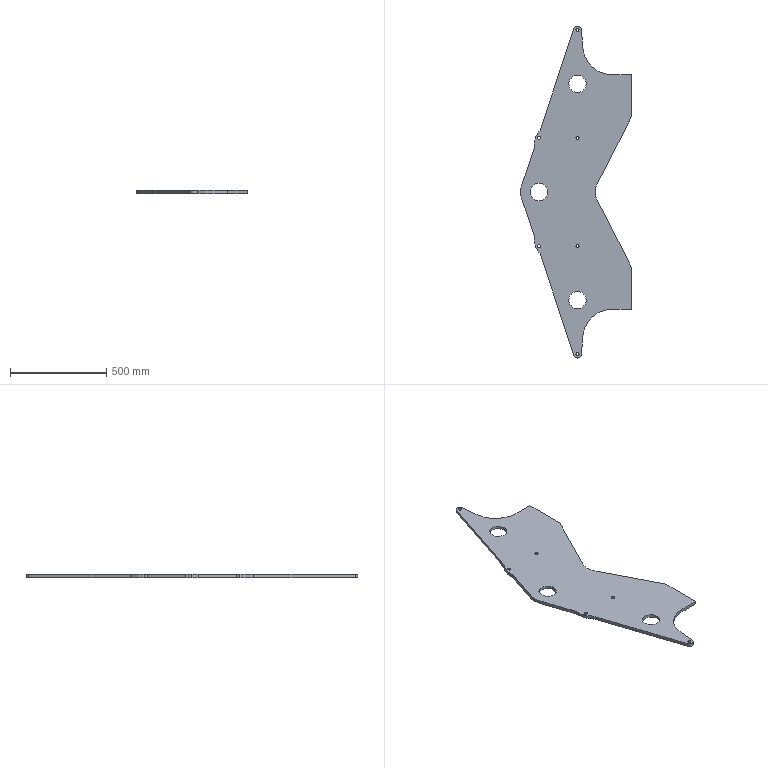Part | SolidWorks | features Extrusion 1, HoleWzd 1, ICE 1 | 1 solid | 44 faces | box 575.631 x 1726 x 16 mm | volume 8635461 mm3 | cylinder 30 | plane 14 | commonest cylinder face diameters 16 x12 200 x8 90 x6 40 x2 300 x2
STEP:
#1=CARTESIAN_POINT('',(-503.404,233.68,16.));
#2=VERTEX_POINT('',#1);
#3=CARTESIAN_POINT('',(-504.662,249.486,16.));
#4=VERTEX_POINT('',#3);
#5=CARTESIAN_POINT('',(-404.662,249.486,16.));
#6=DIRECTION('',(0.,0.,-1.));
#7=DIRECTION('',(1.,0.,0.));
#8=AXIS2_PLACEMENT_3D('',#5,#6,#7);
#9=CIRCLE('',#8,100.);
#10=EDGE_CURVE('',#2,#4,#9,.T.);
#11=ORIENTED_EDGE('',*,*,#10,.T.);
#12=CARTESIAN_POINT('',(-504.662,249.486,0.));
#13=VERTEX_POINT('',#12);
#14=CARTESIAN_POINT('',(-504.662,249.486,16.));
#15=DIRECTION('',(0.,0.,-1.));
#16=VECTOR('',#15,1000.);
#17=LINE('',#14,#16);
#18=EDGE_CURVE('',#4,#13,#17,.T.);
#19=ORIENTED_EDGE('',*,*,#18,.T.);
#20=CARTESIAN_POINT('',(-503.404,233.68,0.));
#21=VERTEX_POINT('',#20);
#22=CARTESIAN_POINT('',(-404.662,249.486,0.));
#23=DIRECTION('',(0.,0.,-1.));
#24=DIRECTION('',(1.,0.,0.));
#25=AXIS2_PLACEMENT_3D('',#22,#23,#24);
#26=CIRCLE('',#25,100.);
#27=EDGE_CURVE('',#21,#13,#26,.T.);
#28=ORIENTED_EDGE('',*,*,#27,.F.);
#29=CARTESIAN_POINT('',(-503.404,233.68,16.));
#30=DIRECTION('',(0.,0.,-1.));
#31=VECTOR('',#30,1000.);
#32=LINE('',#29,#31);
#33=EDGE_CURVE('',#2,#21,#32,.T.);
#34=ORIENTED_EDGE('',*,*,#33,.F.);
#35=EDGE_LOOP('',(#11,#19,#28,#34));
#36=FACE_OUTER_BOUND('',#35,.T.);
#37=CARTESIAN_POINT('',(-404.662,249.486,16.));
#38=DIRECTION('',(0.,0.,-1.));
#39=DIRECTION('',(-1.,0.,0.));
#40=AXIS2_PLACEMENT_3D('',#37,#38,#39);
#41=CYLINDRICAL_SURFACE('',#40,100.);
#42=ADVANCED_FACE('',(#36),#41,.T.);
#43=CARTESIAN_POINT('',(-235.,562.,16.));
#44=VERTEX_POINT('',#43);
#45=CARTESIAN_POINT('',(-325.,562.,16.));
#46=VERTEX_POINT('',#45);
#47=CARTESIAN_POINT('',(-280.,562.,16.));
#48=DIRECTION('',(0.,0.,-1.));
#49=DIRECTION('',(1.,0.,0.));
#50=AXIS2_PLACEMENT_3D('',#47,#48,#49);
#51=CIRCLE('',#50,45.);
#52=EDGE_CURVE('',#44,#46,#51,.T.);
#53=ORIENTED_EDGE('',*,*,#52,.F.);
#54=CARTESIAN_POINT('',(-235.,562.,0.));
#55=VERTEX_POINT('',#54);
#56=CARTESIAN_POINT('',(-235.,562.,16.));
#57=DIRECTION('',(0.,0.,-1.));
#58=VECTOR('',#57,1000.);
#59=LINE('',#56,#58);
#60=EDGE_CURVE('',#44,#55,#59,.T.);
#61=ORIENTED_EDGE('',*,*,#60,.T.);
#62=CARTESIAN_POINT('',(-325.,562.,0.));
#63=VERTEX_POINT('',#62);
#64=CARTESIAN_POINT('',(-280.,562.,0.));
#65=DIRECTION('',(0.,0.,-1.));
#66=DIRECTION('',(1.,0.,0.));
#67=AXIS2_PLACEMENT_3D('',#64,#65,#66);
#68=CIRCLE('',#67,45.);
#69=EDGE_CURVE('',#55,#63,#68,.T.);
#70=ORIENTED_EDGE('',*,*,#69,.T.);
#71=CARTESIAN_POINT('',(-325.,562.,16.));
#72=DIRECTION('',(0.,0.,-1.));
#73=VECTOR('',#72,1000.);
#74=LINE('',#71,#73);
#75=EDGE_CURVE('',#46,#63,#74,.T.);
#76=ORIENTED_EDGE('',*,*,#75,.F.);
#77=EDGE_LOOP('',(#53,#61,#70,#76));
#78=FACE_OUTER_BOUND('',#77,.T.);
#79=CARTESIAN_POINT('',(-280.,562.,16.));
#80=DIRECTION('',(0.,0.,-1.));
#81=DIRECTION('',(-1.,0.,0.));
#82=AXIS2_PLACEMENT_3D('',#79,#80,#81);
#83=CYLINDRICAL_SURFACE('',#82,45.);
#84=ADVANCED_FACE('',(#78),#83,.F.);
#85=CARTESIAN_POINT('',(-272.,281.,16.));
#86=VERTEX_POINT('',#85);
#87=CARTESIAN_POINT('',(-288.,281.,16.));
#88=VERTEX_POINT('',#87);
#89=CARTESIAN_POINT('',(-280.,281.,16.));
#90=DIRECTION('',(0.,0.,-1.));
#91=DIRECTION('',(1.,0.,0.));
#92=AXIS2_PLACEMENT_3D('',#89,#90,#91);
#93=CIRCLE('',#92,8.);
#94=EDGE_CURVE('',#86,#88,#93,.T.);
#95=ORIENTED_EDGE('',*,*,#94,.F.);
#96=CARTESIAN_POINT('',(-272.,281.,0.));
#97=VERTEX_POINT('',#96);
#98=CARTESIAN_POINT('',(-272.,281.,16.));
#99=DIRECTION('',(0.,0.,-1.));
#100=VECTOR('',#99,1000.);
#101=LINE('',#98,#100);
#102=EDGE_CURVE('',#86,#97,#101,.T.);
#103=ORIENTED_EDGE('',*,*,#102,.T.);
#104=CARTESIAN_POINT('',(-288.,281.,0.));
#105=VERTEX_POINT('',#104);
#106=CARTESIAN_POINT('',(-280.,281.,0.));
#107=DIRECTION('',(0.,0.,-1.));
#108=DIRECTION('',(1.,0.,0.));
#109=AXIS2_PLACEMENT_3D('',#106,#107,#108);
#110=CIRCLE('',#109,8.);
#111=EDGE_CURVE('',#97,#105,#110,.T.);
#112=ORIENTED_EDGE('',*,*,#111,.T.);
#113=CARTESIAN_POINT('',(-288.,281.,16.));
#114=DIRECTION('',(0.,0.,-1.));
#115=VECTOR('',#114,1000.);
#116=LINE('',#113,#115);
#117=EDGE_CURVE('',#88,#105,#116,.T.);
#118=ORIENTED_EDGE('',*,*,#117,.F.);
#119=EDGE_LOOP('',(#95,#103,#112,#118));
#120=FACE_OUTER_BOUND('',#119,.T.);
#121=CARTESIAN_POINT('',(-280.,281.,16.));
#122=DIRECTION('',(0.,0.,-1.));
#123=DIRECTION('',(-1.,0.,0.));
#124=AXIS2_PLACEMENT_3D('',#121,#122,#123);
#125=CYLINDRICAL_SURFACE('',#124,8.);
#126=ADVANCED_FACE('',(#120),#125,.F.);
#127=CARTESIAN_POINT('',(-288.,843.,16.));
#128=VERTEX_POINT('',#127);
#129=CARTESIAN_POINT('',(-272.,843.,16.));
#130=VERTEX_POINT('',#129);
#131=CARTESIAN_POINT('',(-280.,843.,16.));
#132=DIRECTION('',(0.,0.,1.));
#133=DIRECTION('',(1.,0.,0.));
#134=AXIS2_PLACEMENT_3D('',#131,#132,#133);
#135=CIRCLE('',#134,8.);
#136=EDGE_CURVE('',#128,#130,#135,.T.);
#137=ORIENTED_EDGE('',*,*,#136,.T.);
#138=CARTESIAN_POINT('',(-272.,843.,0.));
#139=VERTEX_POINT('',#138);
#140=CARTESIAN_POINT('',(-272.,843.,16.));
#141=DIRECTION('',(0.,0.,-1.));
#142=VECTOR('',#141,1000.);
#143=LINE('',#140,#142);
#144=EDGE_CURVE('',#130,#139,#143,.T.);
#145=ORIENTED_EDGE('',*,*,#144,.T.);
#146=CARTESIAN_POINT('',(-288.,843.,0.));
#147=VERTEX_POINT('',#146);
#148=CARTESIAN_POINT('',(-280.,843.,0.));
#149=DIRECTION('',(0.,0.,1.));
#150=DIRECTION('',(1.,0.,0.));
#151=AXIS2_PLACEMENT_3D('',#148,#149,#150);
#152=CIRCLE('',#151,8.);
#153=EDGE_CURVE('',#147,#139,#152,.T.);
#154=ORIENTED_EDGE('',*,*,#153,.F.);
#155=CARTESIAN_POINT('',(-288.,843.,16.));
#156=DIRECTION('',(0.,0.,-1.));
#157=VECTOR('',#156,1000.);
#158=LINE('',#155,#157);
#159=EDGE_CURVE('',#128,#147,#158,.T.);
#160=ORIENTED_EDGE('',*,*,#159,.F.);
#161=EDGE_LOOP('',(#137,#145,#154,#160));
#162=FACE_OUTER_BOUND('',#161,.T.);
#163=CARTESIAN_POINT('',(-280.,843.,16.));
#164=DIRECTION('',(0.,0.,-1.));
#165=DIRECTION('',(-1.,0.,0.));
#166=AXIS2_PLACEMENT_3D('',#163,#164,#165);
#167=CYLINDRICAL_SURFACE('',#166,8.);
#168=ADVANCED_FACE('',(#162),#167,.F.);
#169=CARTESIAN_POINT('',(-288.,-843.,16.));
#170=VERTEX_POINT('',#169);
#171=CARTESIAN_POINT('',(-272.,-843.,16.));
#172=VERTEX_POINT('',#171);
#173=CARTESIAN_POINT('',(-280.,-843.,16.));
#174=DIRECTION('',(0.,0.,1.));
#175=DIRECTION('',(1.,0.,0.));
#176=AXIS2_PLACEMENT_3D('',#173,#174,#175);
#177=CIRCLE('',#176,8.);
#178=EDGE_CURVE('',#170,#172,#177,.T.);
#179=ORIENTED_EDGE('',*,*,#178,.T.);
#180=CARTESIAN_POINT('',(-272.,-843.,0.));
#181=VERTEX_POINT('',#180);
#182=CARTESIAN_POINT('',(-272.,-843.,16.));
#183=DIRECTION('',(0.,0.,-1.));
#184=VECTOR('',#183,1000.);
#185=LINE('',#182,#184);
#186=EDGE_CURVE('',#172,#181,#185,.T.);
#187=ORIENTED_EDGE('',*,*,#186,.T.);
#188=CARTESIAN_POINT('',(-288.,-843.,0.));
#189=VERTEX_POINT('',#188);
#190=CARTESIAN_POINT('',(-280.,-843.,0.));
#191=DIRECTION('',(0.,0.,1.));
#192=DIRECTION('',(1.,0.,0.));
#193=AXIS2_PLACEMENT_3D('',#190,#191,#192);
#194=CIRCLE('',#193,8.);
#195=EDGE_CURVE('',#189,#181,#194,.T.);
#196=ORIENTED_EDGE('',*,*,#195,.F.);
#197=CARTESIAN_POINT('',(-288.,-843.,16.));
#198=DIRECTION('',(0.,0.,-1.));
#199=VECTOR('',#198,1000.);
#200=LINE('',#197,#199);
#201=EDGE_CURVE('',#170,#189,#200,.T.);
#202=ORIENTED_EDGE('',*,*,#201,.F.);
#203=EDGE_LOOP('',(#179,#187,#196,#202));
#204=FACE_OUTER_BOUND('',#203,.T.);
#205=CARTESIAN_POINT('',(-280.,-843.,16.));
#206=DIRECTION('',(0.,0.,-1.));
#207=DIRECTION('',(-1.,0.,0.));
#208=AXIS2_PLACEMENT_3D('',#205,#206,#207);
#209=CYLINDRICAL_SURFACE('',#208,8.);
#210=ADVANCED_FACE('',(#204),#209,.F.);
#211=CARTESIAN_POINT('',(-288.,-281.,16.));
#212=VERTEX_POINT('',#211);
#213=CARTESIAN_POINT('',(-272.,-281.,16.));
#214=VERTEX_POINT('',#213);
#215=CARTESIAN_POINT('',(-280.,-281.,16.));
#216=DIRECTION('',(0.,0.,1.));
#217=DIRECTION('',(1.,0.,0.));
#218=AXIS2_PLACEMENT_3D('',#215,#216,#217);
#219=CIRCLE('',#218,8.);
#220=EDGE_CURVE('',#212,#214,#219,.T.);
#221=ORIENTED_EDGE('',*,*,#220,.T.);
#222=CARTESIAN_POINT('',(-272.,-281.,0.));
#223=VERTEX_POINT('',#222);
#224=CARTESIAN_POINT('',(-272.,-281.,16.));
#225=DIRECTION('',(0.,0.,-1.));
#226=VECTOR('',#225,1000.);
#227=LINE('',#224,#226);
#228=EDGE_CURVE('',#214,#223,#227,.T.);
#229=ORIENTED_EDGE('',*,*,#228,.T.);
#230=CARTESIAN_POINT('',(-288.,-281.,0.));
#231=VERTEX_POINT('',#230);
#232=CARTESIAN_POINT('',(-280.,-281.,0.));
#233=DIRECTION('',(0.,0.,1.));
#234=DIRECTION('',(1.,0.,0.));
#235=AXIS2_PLACEMENT_3D('',#232,#233,#234);
#236=CIRCLE('',#235,8.);
#237=EDGE_CURVE('',#231,#223,#236,.T.);
#238=ORIENTED_EDGE('',*,*,#237,.F.);
#239=CARTESIAN_POINT('',(-288.,-281.,16.));
#240=DIRECTION('',(0.,0.,-1.));
#241=VECTOR('',#240,1000.);
#242=LINE('',#239,#241);
#243=EDGE_CURVE('',#212,#231,#242,.T.);
#244=ORIENTED_EDGE('',*,*,#243,.F.);
#245=EDGE_LOOP('',(#221,#229,#238,#244));
#246=FACE_OUTER_BOUND('',#245,.T.);
#247=CARTESIAN_POINT('',(-280.,-281.,16.));
#248=DIRECTION('',(0.,0.,-1.));
#249=DIRECTION('',(-1.,0.,0.));
#250=AXIS2_PLACEMENT_3D('',#247,#248,#249);
#251=CYLINDRICAL_SURFACE('',#250,8.);
#252=ADVANCED_FACE('',(#246),#251,.F.);
#253=CARTESIAN_POINT('',(-488.,-281.,16.));
#254=VERTEX_POINT('',#253);
#255=CARTESIAN_POINT('',(-472.,-281.,16.));
#256=VERTEX_POINT('',#255);
#257=CARTESIAN_POINT('',(-480.,-281.,16.));
#258=DIRECTION('',(0.,0.,1.));
#259=DIRECTION('',(1.,0.,0.));
#260=AXIS2_PLACEMENT_3D('',#257,#258,#259);
#261=CIRCLE('',#260,8.);
#262=EDGE_CURVE('',#254,#256,#261,.T.);
#263=ORIENTED_EDGE('',*,*,#262,.T.);
#264=CARTESIAN_POINT('',(-472.,-281.,0.));
#265=VERTEX_POINT('',#264);
#266=CARTESIAN_POINT('',(-472.,-281.,16.));
#267=DIRECTION('',(0.,0.,-1.));
#268=VECTOR('',#267,1000.);
#269=LINE('',#266,#268);
#270=EDGE_CURVE('',#256,#265,#269,.T.);
#271=ORIENTED_EDGE('',*,*,#270,.T.);
#272=CARTESIAN_POINT('',(-488.,-281.,0.));
#273=VERTEX_POINT('',#272);
#274=CARTESIAN_POINT('',(-480.,-281.,0.));
#275=DIRECTION('',(0.,0.,1.));
#276=DIRECTION('',(1.,0.,0.));
#277=AXIS2_PLACEMENT_3D('',#274,#275,#276);
#278=CIRCLE('',#277,8.);
#279=EDGE_CURVE('',#273,#265,#278,.T.);
#280=ORIENTED_EDGE('',*,*,#279,.F.);
#281=CARTESIAN_POINT('',(-488.,-281.,16.));
#282=DIRECTION('',(0.,0.,-1.));
#283=VECTOR('',#282,1000.);
#284=LINE('',#281,#283);
#285=EDGE_CURVE('',#254,#273,#284,.T.);
#286=ORIENTED_EDGE('',*,*,#285,.F.);
#287=EDGE_LOOP('',(#263,#271,#280,#286));
#288=FACE_OUTER_BOUND('',#287,.T.);
#289=CARTESIAN_POINT('',(-480.,-281.,16.));
#290=DIRECTION('',(0.,0.,-1.));
#291=DIRECTION('',(-1.,0.,0.));
#292=AXIS2_PLACEMENT_3D('',#289,#290,#291);
#293=CYLINDRICAL_SURFACE('',#292,8.);
#294=ADVANCED_FACE('',(#288),#293,.F.);
#295=CARTESIAN_POINT('',(-325.,-562.,16.));
#296=VERTEX_POINT('',#295);
#297=CARTESIAN_POINT('',(-235.,-562.,16.));
#298=VERTEX_POINT('',#297);
#299=CARTESIAN_POINT('',(-280.,-562.,16.));
#300=DIRECTION('',(0.,0.,1.));
#301=DIRECTION('',(1.,0.,0.));
#302=AXIS2_PLACEMENT_3D('',#299,#300,#301);
#303=CIRCLE('',#302,45.);
#304=EDGE_CURVE('',#296,#298,#303,.T.);
#305=ORIENTED_EDGE('',*,*,#304,.T.);
#306=CARTESIAN_POINT('',(-235.,-562.,0.));
#307=VERTEX_POINT('',#306);
#308=CARTESIAN_POINT('',(-235.,-562.,16.));
#309=DIRECTION('',(0.,0.,-1.));
#310=VECTOR('',#309,1000.);
#311=LINE('',#308,#310);
#312=EDGE_CURVE('',#298,#307,#311,.T.);
#313=ORIENTED_EDGE('',*,*,#312,.T.);
#314=CARTESIAN_POINT('',(-325.,-562.,0.));
#315=VERTEX_POINT('',#314);
#316=CARTESIAN_POINT('',(-280.,-562.,0.));
#317=DIRECTION('',(0.,0.,1.));
#318=DIRECTION('',(1.,0.,0.));
#319=AXIS2_PLACEMENT_3D('',#316,#317,#318);
#320=CIRCLE('',#319,45.);
#321=EDGE_CURVE('',#315,#307,#320,.T.);
#322=ORIENTED_EDGE('',*,*,#321,.F.);
#323=CARTESIAN_POINT('',(-325.,-562.,16.));
#324=DIRECTION('',(0.,0.,-1.));
#325=VECTOR('',#324,1000.);
#326=LINE('',#323,#325);
#327=EDGE_CURVE('',#296,#315,#326,.T.);
#328=ORIENTED_EDGE('',*,*,#327,.F.);
#329=EDGE_LOOP('',(#305,#313,#322,#328));
#330=FACE_OUTER_BOUND('',#329,.T.);
#331=CARTESIAN_POINT('',(-280.,-562.,16.));
#332=DIRECTION('',(0.,0.,-1.));
#333=DIRECTION('',(-1.,0.,0.));
#334=AXIS2_PLACEMENT_3D('',#331,#332,#333);
#335=CYLINDRICAL_SURFACE('',#334,45.);
#336=ADVANCED_FACE('',(#330),#335,.F.);
#337=CARTESIAN_POINT('',(-525.,0.,16.));
#338=VERTEX_POINT('',#337);
#339=CARTESIAN_POINT('',(-435.,0.,16.));
#340=VERTEX_POINT('',#339);
#341=CARTESIAN_POINT('',(-480.,0.,16.));
#342=DIRECTION('',(0.,0.,1.));
#343=DIRECTION('',(1.,0.,0.));
#344=AXIS2_PLACEMENT_3D('',#341,#342,#343);
#345=CIRCLE('',#344,45.);
#346=EDGE_CURVE('',#338,#340,#345,.T.);
#347=ORIENTED_EDGE('',*,*,#346,.T.);
#348=CARTESIAN_POINT('',(-435.,0.,0.));
#349=VERTEX_POINT('',#348);
#350=CARTESIAN_POINT('',(-435.,0.,16.));
#351=DIRECTION('',(0.,0.,-1.));
#352=VECTOR('',#351,1000.);
#353=LINE('',#350,#352);
#354=EDGE_CURVE('',#340,#349,#353,.T.);
#355=ORIENTED_EDGE('',*,*,#354,.T.);
#356=CARTESIAN_POINT('',(-525.,0.,0.));
#357=VERTEX_POINT('',#356);
#358=CARTESIAN_POINT('',(-480.,0.,0.));
#359=DIRECTION('',(0.,0.,1.));
#360=DIRECTION('',(1.,0.,0.));
#361=AXIS2_PLACEMENT_3D('',#358,#359,#360);
#362=CIRCLE('',#361,45.);
#363=EDGE_CURVE('',#357,#349,#362,.T.);
#364=ORIENTED_EDGE('',*,*,#363,.F.);
#365=CARTESIAN_POINT('',(-525.,0.,16.));
#366=DIRECTION('',(0.,0.,-1.));
#367=VECTOR('',#366,1000.);
#368=LINE('',#365,#367);
#369=EDGE_CURVE('',#338,#357,#368,.T.);
#370=ORIENTED_EDGE('',*,*,#369,.F.);
#371=EDGE_LOOP('',(#347,#355,#364,#370));
#372=FACE_OUTER_BOUND('',#371,.T.);
#373=CARTESIAN_POINT('',(-480.,0.,16.));
#374=DIRECTION('',(0.,0.,-1.));
#375=DIRECTION('',(-1.,0.,0.));
#376=AXIS2_PLACEMENT_3D('',#373,#374,#375);
#377=CYLINDRICAL_SURFACE('',#376,45.);
#378=ADVANCED_FACE('',(#372),#377,.F.);
#379=CARTESIAN_POINT('',(-472.,281.,16.));
#380=VERTEX_POINT('',#379);
#381=CARTESIAN_POINT('',(-488.,281.,16.));
#382=VERTEX_POINT('',#381);
#383=CARTESIAN_POINT('',(-480.,281.,16.));
#384=DIRECTION('',(0.,0.,-1.));
#385=DIRECTION('',(1.,0.,0.));
#386=AXIS2_PLACEMENT_3D('',#383,#384,#385);
#387=CIRCLE('',#386,8.);
#388=EDGE_CURVE('',#380,#382,#387,.T.);
#389=ORIENTED_EDGE('',*,*,#388,.F.);
#390=CARTESIAN_POINT('',(-472.,281.,0.));
#391=VERTEX_POINT('',#390);
#392=CARTESIAN_POINT('',(-472.,281.,16.));
#393=DIRECTION('',(0.,0.,-1.));
#394=VECTOR('',#393,1000.);
#395=LINE('',#392,#394);
#396=EDGE_CURVE('',#380,#391,#395,.T.);
#397=ORIENTED_EDGE('',*,*,#396,.T.);
#398=CARTESIAN_POINT('',(-488.,281.,0.));
#399=VERTEX_POINT('',#398);
#400=CARTESIAN_POINT('',(-480.,281.,0.));
#401=DIRECTION('',(0.,0.,-1.));
#402=DIRECTION('',(1.,0.,0.));
#403=AXIS2_PLACEMENT_3D('',#400,#401,#402);
#404=CIRCLE('',#403,8.);
#405=EDGE_CURVE('',#391,#399,#404,.T.);
#406=ORIENTED_EDGE('',*,*,#405,.T.);
#407=CARTESIAN_POINT('',(-488.,281.,16.));
#408=DIRECTION('',(0.,0.,-1.));
#409=VECTOR('',#408,1000.);
#410=LINE('',#407,#409);
#411=EDGE_CURVE('',#382,#399,#410,.T.);
#412=ORIENTED_EDGE('',*,*,#411,.F.);
#413=EDGE_LOOP('',(#389,#397,#406,#412));
#414=FACE_OUTER_BOUND('',#413,.T.);
#415=CARTESIAN_POINT('',(-480.,281.,16.));
#416=DIRECTION('',(0.,0.,-1.));
#417=DIRECTION('',(-1.,0.,0.));
#418=AXIS2_PLACEMENT_3D('',#415,#416,#417);
#419=CYLINDRICAL_SURFACE('',#418,8.);
#420=ADVANCED_FACE('',(#414),#419,.F.);
#421=CARTESIAN_POINT('',(-176.599,45.632,16.));
#422=VERTEX_POINT('',#421);
#423=CARTESIAN_POINT('',(-187.617,0.,16.));
#424=VERTEX_POINT('',#423);
#425=CARTESIAN_POINT('',(-87.617,0.,16.));
#426=DIRECTION('',(0.,0.,1.));
#427=DIRECTION('',(1.,0.,0.));
#428=AXIS2_PLACEMENT_3D('',#425,#426,#427);
#429=CIRCLE('',#428,100.);
#430=EDGE_CURVE('',#422,#424,#429,.T.);
#431=ORIENTED_EDGE('',*,*,#430,.T.);
#432=CARTESIAN_POINT('',(-187.617,0.,0.));
#433=VERTEX_POINT('',#432);
#434=CARTESIAN_POINT('',(-187.617,0.,16.));
#435=DIRECTION('',(0.,0.,-1.));
#436=VECTOR('',#435,1000.);
#437=LINE('',#434,#436);
#438=EDGE_CURVE('',#424,#433,#437,.T.);
#439=ORIENTED_EDGE('',*,*,#438,.T.);
#440=CARTESIAN_POINT('',(-176.599,45.632,0.));
#441=VERTEX_POINT('',#440);
#442=CARTESIAN_POINT('',(-87.617,0.,0.));
#443=DIRECTION('',(0.,0.,1.));
#444=DIRECTION('',(1.,0.,0.));
#445=AXIS2_PLACEMENT_3D('',#442,#443,#444);
#446=CIRCLE('',#445,100.);
#447=EDGE_CURVE('',#441,#433,#446,.T.);
#448=ORIENTED_EDGE('',*,*,#447,.F.);
#449=CARTESIAN_POINT('',(-176.599,45.632,16.));
#450=DIRECTION('',(0.,0.,-1.));
#451=VECTOR('',#450,1000.);
#452=LINE('',#449,#451);
#453=EDGE_CURVE('',#422,#441,#452,.T.);
#454=ORIENTED_EDGE('',*,*,#453,.F.);
#455=EDGE_LOOP('',(#431,#439,#448,#454));
#456=FACE_OUTER_BOUND('',#455,.T.);
#457=CARTESIAN_POINT('',(-87.617,0.,16.));
#458=DIRECTION('',(0.,0.,-1.));
#459=DIRECTION('',(-1.,0.,0.));
#460=AXIS2_PLACEMENT_3D('',#457,#458,#459);
#461=CYLINDRICAL_SURFACE('',#460,100.);
#462=ADVANCED_FACE('',(#456),#461,.F.);
#463=CARTESIAN_POINT('',(-504.662,-249.486,16.));
#464=VERTEX_POINT('',#463);
#465=CARTESIAN_POINT('',(-474.337,-321.217,16.));
#466=VERTEX_POINT('',#465);
#467=CARTESIAN_POINT('',(-404.662,-249.486,16.));
#468=DIRECTION('',(0.,0.,1.));
#469=DIRECTION('',(1.,0.,0.));
#470=AXIS2_PLACEMENT_3D('',#467,#468,#469);
#471=CIRCLE('',#470,100.);
#472=EDGE_CURVE('',#464,#466,#471,.T.);
#473=ORIENTED_EDGE('',*,*,#472,.F.);
#474=CARTESIAN_POINT('',(-504.662,-249.486,0.));
#475=VERTEX_POINT('',#474);
#476=CARTESIAN_POINT('',(-504.662,-249.486,16.));
#477=DIRECTION('',(0.,0.,-1.));
#478=VECTOR('',#477,1000.);
#479=LINE('',#476,#478);
#480=EDGE_CURVE('',#464,#475,#479,.T.);
#481=ORIENTED_EDGE('',*,*,#480,.T.);
#482=CARTESIAN_POINT('',(-474.337,-321.217,0.));
#483=VERTEX_POINT('',#482);
#484=CARTESIAN_POINT('',(-404.662,-249.486,0.));
#485=DIRECTION('',(0.,0.,1.));
#486=DIRECTION('',(1.,0.,0.));
#487=AXIS2_PLACEMENT_3D('',#484,#485,#486);
#488=CIRCLE('',#487,100.);
#489=EDGE_CURVE('',#475,#483,#488,.T.);
#490=ORIENTED_EDGE('',*,*,#489,.T.);
#491=CARTESIAN_POINT('',(-474.337,-321.217,16.));
#492=DIRECTION('',(0.,0.,-1.));
#493=VECTOR('',#492,1000.);
#494=LINE('',#491,#493);
#495=EDGE_CURVE('',#466,#483,#494,.T.);
#496=ORIENTED_EDGE('',*,*,#495,.F.);
#497=EDGE_LOOP('',(#473,#481,#490,#496));
#498=FACE_OUTER_BOUND('',#497,.T.);
#499=CARTESIAN_POINT('',(-404.662,-249.486,16.));
#500=DIRECTION('',(0.,0.,-1.));
#501=DIRECTION('',(-1.,0.,0.));
#502=AXIS2_PLACEMENT_3D('',#499,#500,#501);
#503=CYLINDRICAL_SURFACE('',#502,100.);
#504=ADVANCED_FACE('',(#498),#503,.T.);
#505=CARTESIAN_POINT('',(-575.631,0.,16.));
#506=VERTEX_POINT('',#505);
#507=CARTESIAN_POINT('',(-570.535,-31.514,16.));
#508=VERTEX_POINT('',#507);
#509=CARTESIAN_POINT('',(-475.631,0.,16.));
#510=DIRECTION('',(0.,0.,1.));
#511=DIRECTION('',(1.,0.,0.));
#512=AXIS2_PLACEMENT_3D('',#509,#510,#511);
#513=CIRCLE('',#512,100.);
#514=EDGE_CURVE('',#506,#508,#513,.T.);
#515=ORIENTED_EDGE('',*,*,#514,.F.);
#516=CARTESIAN_POINT('',(-575.631,0.,0.));
#517=VERTEX_POINT('',#516);
#518=CARTESIAN_POINT('',(-575.631,0.,16.));
#519=DIRECTION('',(0.,0.,-1.));
#520=VECTOR('',#519,1000.);
#521=LINE('',#518,#520);
#522=EDGE_CURVE('',#506,#517,#521,.T.);
#523=ORIENTED_EDGE('',*,*,#522,.T.);
#524=CARTESIAN_POINT('',(-570.535,-31.514,0.));
#525=VERTEX_POINT('',#524);
#526=CARTESIAN_POINT('',(-475.631,0.,0.));
#527=DIRECTION('',(0.,0.,1.));
#528=DIRECTION('',(1.,0.,0.));
#529=AXIS2_PLACEMENT_3D('',#526,#527,#528);
#530=CIRCLE('',#529,100.);
#531=EDGE_CURVE('',#517,#525,#530,.T.);
#532=ORIENTED_EDGE('',*,*,#531,.T.);
#533=CARTESIAN_POINT('',(-570.535,-31.514,16.));
#534=DIRECTION('',(0.,0.,-1.));
#535=VECTOR('',#534,1000.);
#536=LINE('',#533,#535);
#537=EDGE_CURVE('',#508,#525,#536,.T.);
#538=ORIENTED_EDGE('',*,*,#537,.F.);
#539=EDGE_LOOP('',(#515,#523,#532,#538));
#540=FACE_OUTER_BOUND('',#539,.T.);
#541=CARTESIAN_POINT('',(-475.631,0.,16.));
#542=DIRECTION('',(0.,0.,-1.));
#543=DIRECTION('',(-1.,0.,0.));
#544=AXIS2_PLACEMENT_3D('',#541,#542,#543);
#545=CYLINDRICAL_SURFACE('',#544,100.);
#546=ADVANCED_FACE('',(#540),#545,.T.);
#547=CARTESIAN_POINT('',(-570.535,31.514,0.));
#548=VERTEX_POINT('',#547);
#549=CARTESIAN_POINT('',(-523.299,173.766,0.));
#550=DIRECTION('',(0.3151,0.949,0.));
#551=VECTOR('',#550,1000.);
#552=LINE('',#549,#551);
#553=EDGE_CURVE('',#548,#21,#552,.T.);
#554=ORIENTED_EDGE('',*,*,#553,.F.);
#555=CARTESIAN_POINT('',(-570.535,31.514,16.));
#556=VERTEX_POINT('',#555);
#557=CARTESIAN_POINT('',(-570.535,31.514,16.));
#558=DIRECTION('',(0.,0.,-1.));
#559=VECTOR('',#558,1000.);
#560=LINE('',#557,#559);
#561=EDGE_CURVE('',#556,#548,#560,.T.);
#562=ORIENTED_EDGE('',*,*,#561,.F.);
#563=CARTESIAN_POINT('',(-523.299,173.766,16.));
#564=DIRECTION('',(0.3151,0.949,0.));
#565=VECTOR('',#564,1000.);
#566=LINE('',#563,#565);
#567=EDGE_CURVE('',#556,#2,#566,.T.);
#568=ORIENTED_EDGE('',*,*,#567,.T.);
#569=ORIENTED_EDGE('',*,*,#33,.T.);
#570=EDGE_LOOP('',(#554,#562,#568,#569));
#571=FACE_OUTER_BOUND('',#570,.T.);
#572=CARTESIAN_POINT('',(-523.299,173.766,16.));
#573=DIRECTION('',(-0.949,0.3151,0.));
#574=DIRECTION('',(-0.3151,-0.949,0.));
#575=AXIS2_PLACEMENT_3D('',#572,#573,#574);
#576=PLANE('',#575);
#577=ADVANCED_FACE('',(#571),#576,.T.);
#578=ORIENTED_EDGE('',*,*,#522,.F.);
#579=CARTESIAN_POINT('',(-475.631,0.,16.));
#580=DIRECTION('',(0.,0.,1.));
#581=DIRECTION('',(1.,0.,0.));
#582=AXIS2_PLACEMENT_3D('',#579,#580,#581);
#583=CIRCLE('',#582,100.);
#584=EDGE_CURVE('',#556,#506,#583,.T.);
#585=ORIENTED_EDGE('',*,*,#584,.F.);
#586=ORIENTED_EDGE('',*,*,#561,.T.);
#587=CARTESIAN_POINT('',(-475.631,0.,0.));
#588=DIRECTION('',(0.,0.,1.));
#589=DIRECTION('',(1.,0.,0.));
#590=AXIS2_PLACEMENT_3D('',#587,#588,#589);
#591=CIRCLE('',#590,100.);
#592=EDGE_CURVE('',#548,#517,#591,.T.);
#593=ORIENTED_EDGE('',*,*,#592,.T.);
#594=EDGE_LOOP('',(#578,#585,#586,#593));
#595=FACE_OUTER_BOUND('',#594,.T.);
#596=CARTESIAN_POINT('',(-475.631,0.,16.));
#597=DIRECTION('',(0.,0.,-1.));
#598=DIRECTION('',(-1.,0.,0.));
#599=AXIS2_PLACEMENT_3D('',#596,#597,#598);
#600=CYLINDRICAL_SURFACE('',#599,100.);
#601=ADVANCED_FACE('',(#595),#600,.T.);
#602=CARTESIAN_POINT('',(-503.404,-233.68,0.));
#603=VERTEX_POINT('',#602);
#604=CARTESIAN_POINT('',(-523.299,-173.766,0.));
#605=DIRECTION('',(0.3151,-0.949,0.));
#606=VECTOR('',#605,1000.);
#607=LINE('',#604,#606);
#608=EDGE_CURVE('',#525,#603,#607,.T.);
#609=ORIENTED_EDGE('',*,*,#608,.T.);
#610=CARTESIAN_POINT('',(-503.404,-233.68,16.));
#611=VERTEX_POINT('',#610);
#612=CARTESIAN_POINT('',(-503.404,-233.68,16.));
#613=DIRECTION('',(0.,0.,-1.));
#614=VECTOR('',#613,1000.);
#615=LINE('',#612,#614);
#616=EDGE_CURVE('',#611,#603,#615,.T.);
#617=ORIENTED_EDGE('',*,*,#616,.F.);
#618=CARTESIAN_POINT('',(-523.299,-173.766,16.));
#619=DIRECTION('',(0.3151,-0.949,0.));
#620=VECTOR('',#619,1000.);
#621=LINE('',#618,#620);
#622=EDGE_CURVE('',#508,#611,#621,.T.);
#623=ORIENTED_EDGE('',*,*,#622,.F.);
#624=ORIENTED_EDGE('',*,*,#537,.T.);
#625=EDGE_LOOP('',(#609,#617,#623,#624));
#626=FACE_OUTER_BOUND('',#625,.T.);
#627=CARTESIAN_POINT('',(-523.299,-173.766,16.));
#628=DIRECTION('',(0.949,0.3151,0.));
#629=DIRECTION('',(-0.3151,0.949,0.));
#630=AXIS2_PLACEMENT_3D('',#627,#628,#629);
#631=PLANE('',#630);
#632=ADVANCED_FACE('',(#626),#631,.F.);
#633=ORIENTED_EDGE('',*,*,#480,.F.);
#634=CARTESIAN_POINT('',(-404.662,-249.486,16.));
#635=DIRECTION('',(0.,0.,1.));
#636=DIRECTION('',(1.,0.,0.));
#637=AXIS2_PLACEMENT_3D('',#634,#635,#636);
#638=CIRCLE('',#637,100.);
#639=EDGE_CURVE('',#611,#464,#638,.T.);
#640=ORIENTED_EDGE('',*,*,#639,.F.);
#641=ORIENTED_EDGE('',*,*,#616,.T.);
#642=CARTESIAN_POINT('',(-404.662,-249.486,0.));
#643=DIRECTION('',(0.,0.,1.));
#644=DIRECTION('',(1.,0.,0.));
#645=AXIS2_PLACEMENT_3D('',#642,#643,#644);
#646=CIRCLE('',#645,100.);
#647=EDGE_CURVE('',#603,#475,#646,.T.);
#648=ORIENTED_EDGE('',*,*,#647,.T.);
#649=EDGE_LOOP('',(#633,#640,#641,#648));
#650=FACE_OUTER_BOUND('',#649,.T.);
#651=CARTESIAN_POINT('',(-404.662,-249.486,16.));
#652=DIRECTION('',(0.,0.,-1.));
#653=DIRECTION('',(-1.,0.,0.));
#654=AXIS2_PLACEMENT_3D('',#651,#652,#653);
#655=CYLINDRICAL_SURFACE('',#654,100.);
#656=ADVANCED_FACE('',(#650),#655,.T.);
#657=CARTESIAN_POINT('',(-298.981,-849.303,0.));
#658=VERTEX_POINT('',#657);
#659=CARTESIAN_POINT('',(-523.299,-173.766,0.));
#660=DIRECTION('',(0.3151,-0.949,0.));
#661=VECTOR('',#660,1000.);
#662=LINE('',#659,#661);
#663=EDGE_CURVE('',#483,#658,#662,.T.);
#664=ORIENTED_EDGE('',*,*,#663,.T.);
#665=CARTESIAN_POINT('',(-298.981,-849.303,16.));
#666=VERTEX_POINT('',#665);
#667=CARTESIAN_POINT('',(-298.981,-849.303,16.));
#668=DIRECTION('',(0.,0.,-1.));
#669=VECTOR('',#668,1000.);
#670=LINE('',#667,#669);
#671=EDGE_CURVE('',#666,#658,#670,.T.);
#672=ORIENTED_EDGE('',*,*,#671,.F.);
#673=CARTESIAN_POINT('',(-523.299,-173.766,16.));
#674=DIRECTION('',(0.3151,-0.949,0.));
#675=VECTOR('',#674,1000.);
#676=LINE('',#673,#675);
#677=EDGE_CURVE('',#466,#666,#676,.T.);
#678=ORIENTED_EDGE('',*,*,#677,.F.);
#679=ORIENTED_EDGE('',*,*,#495,.T.);
#680=EDGE_LOOP('',(#664,#672,#678,#679));
#681=FACE_OUTER_BOUND('',#680,.T.);
#682=CARTESIAN_POINT('',(-523.299,-173.766,16.));
#683=DIRECTION('',(0.949,0.3151,0.));
#684=DIRECTION('',(-0.3151,0.949,0.));
#685=AXIS2_PLACEMENT_3D('',#682,#683,#684);
#686=PLANE('',#685);
#687=ADVANCED_FACE('',(#681),#686,.F.);
#688=CARTESIAN_POINT('',(-260.076,-844.743,0.));
#689=VERTEX_POINT('',#688);
#690=CARTESIAN_POINT('',(-280.,-843.,0.));
#691=DIRECTION('',(0.,0.,-1.));
#692=DIRECTION('',(1.,0.,0.));
#693=AXIS2_PLACEMENT_3D('',#690,#691,#692);
#694=CIRCLE('',#693,20.);
#695=EDGE_CURVE('',#689,#658,#694,.T.);
#696=ORIENTED_EDGE('',*,*,#695,.F.);
#697=CARTESIAN_POINT('',(-260.076,-844.743,16.));
#698=VERTEX_POINT('',#697);
#699=CARTESIAN_POINT('',(-260.076,-844.743,16.));
#700=DIRECTION('',(0.,0.,-1.));
#701=VECTOR('',#700,1000.);
#702=LINE('',#699,#701);
#703=EDGE_CURVE('',#698,#689,#702,.T.);
#704=ORIENTED_EDGE('',*,*,#703,.F.);
#705=CARTESIAN_POINT('',(-280.,-843.,16.));
#706=DIRECTION('',(0.,0.,-1.));
#707=DIRECTION('',(1.,0.,0.));
#708=AXIS2_PLACEMENT_3D('',#705,#706,#707);
#709=CIRCLE('',#708,20.);
#710=EDGE_CURVE('',#698,#666,#709,.T.);
#711=ORIENTED_EDGE('',*,*,#710,.T.);
#712=ORIENTED_EDGE('',*,*,#671,.T.);
#713=EDGE_LOOP('',(#696,#704,#711,#712));
#714=FACE_OUTER_BOUND('',#713,.T.);
#715=CARTESIAN_POINT('',(-280.,-843.,16.));
#716=DIRECTION('',(0.,0.,-1.));
#717=DIRECTION('',(-1.,0.,0.));
#718=AXIS2_PLACEMENT_3D('',#715,#716,#717);
#719=CYLINDRICAL_SURFACE('',#718,20.);
#720=ADVANCED_FACE('',(#714),#719,.T.);
#721=CARTESIAN_POINT('',(-251.518,-746.927,0.));
#722=VERTEX_POINT('',#721);
#723=CARTESIAN_POINT('',(-184.756,16.164,0.));
#724=DIRECTION('',(0.08716,0.9962,0.));
#725=VECTOR('',#724,1000.);
#726=LINE('',#723,#725);
#727=EDGE_CURVE('',#689,#722,#726,.T.);
#728=ORIENTED_EDGE('',*,*,#727,.T.);
#729=CARTESIAN_POINT('',(-251.518,-746.927,16.));
#730=VERTEX_POINT('',#729);
#731=CARTESIAN_POINT('',(-251.518,-746.927,16.));
#732=DIRECTION('',(0.,0.,-1.));
#733=VECTOR('',#732,1000.);
#734=LINE('',#731,#733);
#735=EDGE_CURVE('',#730,#722,#734,.T.);
#736=ORIENTED_EDGE('',*,*,#735,.F.);
#737=CARTESIAN_POINT('',(-184.756,16.164,16.));
#738=DIRECTION('',(0.08716,0.9962,0.));
#739=VECTOR('',#738,1000.);
#740=LINE('',#737,#739);
#741=EDGE_CURVE('',#698,#730,#740,.T.);
#742=ORIENTED_EDGE('',*,*,#741,.F.);
#743=ORIENTED_EDGE('',*,*,#703,.T.);
#744=EDGE_LOOP('',(#728,#736,#742,#743));
#745=FACE_OUTER_BOUND('',#744,.T.);
#746=CARTESIAN_POINT('',(-184.756,16.164,16.));
#747=DIRECTION('',(-0.9962,0.08716,0.));
#748=DIRECTION('',(-0.08716,-0.9962,0.));
#749=AXIS2_PLACEMENT_3D('',#746,#747,#748);
#750=PLANE('',#749);
#751=ADVANCED_FACE('',(#745),#750,.F.);
#752=CARTESIAN_POINT('',(-102.089,-610.,0.));
#753=VERTEX_POINT('',#752);
#754=CARTESIAN_POINT('',(-102.089,-760.,0.));
#755=DIRECTION('',(0.,0.,1.));
#756=DIRECTION('',(1.,0.,0.));
#757=AXIS2_PLACEMENT_3D('',#754,#755,#756);
#758=CIRCLE('',#757,150.);
#759=EDGE_CURVE('',#753,#722,#758,.T.);
#760=ORIENTED_EDGE('',*,*,#759,.F.);
#761=CARTESIAN_POINT('',(-102.089,-610.,16.));
#762=VERTEX_POINT('',#761);
#763=CARTESIAN_POINT('',(-102.089,-610.,16.));
#764=DIRECTION('',(0.,0.,-1.));
#765=VECTOR('',#764,1000.);
#766=LINE('',#763,#765);
#767=EDGE_CURVE('',#762,#753,#766,.T.);
#768=ORIENTED_EDGE('',*,*,#767,.F.);
#769=CARTESIAN_POINT('',(-102.089,-760.,16.));
#770=DIRECTION('',(0.,0.,1.));
#771=DIRECTION('',(1.,0.,0.));
#772=AXIS2_PLACEMENT_3D('',#769,#770,#771);
#773=CIRCLE('',#772,150.);
#774=EDGE_CURVE('',#762,#730,#773,.T.);
#775=ORIENTED_EDGE('',*,*,#774,.T.);
#776=ORIENTED_EDGE('',*,*,#735,.T.);
#777=EDGE_LOOP('',(#760,#768,#775,#776));
#778=FACE_OUTER_BOUND('',#777,.T.);
#779=CARTESIAN_POINT('',(-102.089,-760.,16.));
#780=DIRECTION('',(0.,0.,-1.));
#781=DIRECTION('',(-1.,0.,0.));
#782=AXIS2_PLACEMENT_3D('',#779,#780,#781);
#783=CYLINDRICAL_SURFACE('',#782,150.);
#784=ADVANCED_FACE('',(#778),#783,.F.);
#785=CARTESIAN_POINT('',(0.,-610.,0.));
#786=VERTEX_POINT('',#785);
#787=CARTESIAN_POINT('',(0.,-610.,0.));
#788=DIRECTION('',(1.,0.,0.));
#789=VECTOR('',#788,1000.);
#790=LINE('',#787,#789);
#791=EDGE_CURVE('',#753,#786,#790,.T.);
#792=ORIENTED_EDGE('',*,*,#791,.T.);
#793=CARTESIAN_POINT('',(0.,-610.,16.));
#794=VERTEX_POINT('',#793);
#795=CARTESIAN_POINT('',(0.,-610.,16.));
#796=DIRECTION('',(0.,0.,-1.));
#797=VECTOR('',#796,1000.);
#798=LINE('',#795,#797);
#799=EDGE_CURVE('',#794,#786,#798,.T.);
#800=ORIENTED_EDGE('',*,*,#799,.F.);
#801=CARTESIAN_POINT('',(0.,-610.,16.));
#802=DIRECTION('',(1.,0.,0.));
#803=VECTOR('',#802,1000.);
#804=LINE('',#801,#803);
#805=EDGE_CURVE('',#762,#794,#804,.T.);
#806=ORIENTED_EDGE('',*,*,#805,.F.);
#807=ORIENTED_EDGE('',*,*,#767,.T.);
#808=EDGE_LOOP('',(#792,#800,#806,#807));
#809=FACE_OUTER_BOUND('',#808,.T.);
#810=CARTESIAN_POINT('',(0.,-610.,16.));
#811=DIRECTION('',(0.,1.,0.));
#812=DIRECTION('',(-1.,0.,0.));
#813=AXIS2_PLACEMENT_3D('',#810,#811,#812);
#814=PLANE('',#813);
#815=ADVANCED_FACE('',(#809),#814,.F.);
#816=CARTESIAN_POINT('',(0.,-390.,0.));
#817=VERTEX_POINT('',#816);
#818=CARTESIAN_POINT('',(0.,0.,0.));
#819=DIRECTION('',(0.,-1.,0.));
#820=VECTOR('',#819,1000.);
#821=LINE('',#818,#820);
#822=EDGE_CURVE('',#817,#786,#821,.T.);
#823=ORIENTED_EDGE('',*,*,#822,.F.);
#824=CARTESIAN_POINT('',(0.,-390.,16.));
#825=VERTEX_POINT('',#824);
#826=CARTESIAN_POINT('',(0.,-390.,16.));
#827=DIRECTION('',(0.,0.,-1.));
#828=VECTOR('',#827,1000.);
#829=LINE('',#826,#828);
#830=EDGE_CURVE('',#825,#817,#829,.T.);
#831=ORIENTED_EDGE('',*,*,#830,.F.);
#832=CARTESIAN_POINT('',(0.,0.,16.));
#833=DIRECTION('',(0.,-1.,0.));
#834=VECTOR('',#833,1000.);
#835=LINE('',#832,#834);
#836=EDGE_CURVE('',#825,#794,#835,.T.);
#837=ORIENTED_EDGE('',*,*,#836,.T.);
#838=ORIENTED_EDGE('',*,*,#799,.T.);
#839=EDGE_LOOP('',(#823,#831,#837,#838));
#840=FACE_OUTER_BOUND('',#839,.T.);
#841=CARTESIAN_POINT('',(0.,0.,16.));
#842=DIRECTION('',(1.,0.,0.));
#843=DIRECTION('',(0.,1.,0.));
#844=AXIS2_PLACEMENT_3D('',#841,#842,#843);
#845=PLANE('',#844);
#846=ADVANCED_FACE('',(#840),#845,.T.);
#847=CARTESIAN_POINT('',(-176.599,-45.632,0.));
#848=VERTEX_POINT('',#847);
#849=CARTESIAN_POINT('',(-158.355,-81.208,0.));
#850=DIRECTION('',(0.4563,-0.8898,0.));
#851=VECTOR('',#850,1000.);
#852=LINE('',#849,#851);
#853=EDGE_CURVE('',#848,#817,#852,.T.);
#854=ORIENTED_EDGE('',*,*,#853,.F.);
#855=CARTESIAN_POINT('',(-176.599,-45.632,16.));
#856=VERTEX_POINT('',#855);
#857=CARTESIAN_POINT('',(-176.599,-45.632,16.));
#858=DIRECTION('',(0.,0.,-1.));
#859=VECTOR('',#858,1000.);
#860=LINE('',#857,#859);
#861=EDGE_CURVE('',#856,#848,#860,.T.);
#862=ORIENTED_EDGE('',*,*,#861,.F.);
#863=CARTESIAN_POINT('',(-158.355,-81.208,16.));
#864=DIRECTION('',(0.4563,-0.8898,0.));
#865=VECTOR('',#864,1000.);
#866=LINE('',#863,#865);
#867=EDGE_CURVE('',#856,#825,#866,.T.);
#868=ORIENTED_EDGE('',*,*,#867,.T.);
#869=ORIENTED_EDGE('',*,*,#830,.T.);
#870=EDGE_LOOP('',(#854,#862,#868,#869));
#871=FACE_OUTER_BOUND('',#870,.T.);
#872=CARTESIAN_POINT('',(-158.355,-81.208,16.));
#873=DIRECTION('',(0.8898,0.4563,0.));
#874=DIRECTION('',(-0.4563,0.8898,0.));
#875=AXIS2_PLACEMENT_3D('',#872,#873,#874);
#876=PLANE('',#875);
#877=ADVANCED_FACE('',(#871),#876,.T.);
#878=ORIENTED_EDGE('',*,*,#438,.F.);
#879=CARTESIAN_POINT('',(-87.617,0.,16.));
#880=DIRECTION('',(0.,0.,1.));
#881=DIRECTION('',(1.,0.,0.));
#882=AXIS2_PLACEMENT_3D('',#879,#880,#881);
#883=CIRCLE('',#882,100.);
#884=EDGE_CURVE('',#424,#856,#883,.T.);
#885=ORIENTED_EDGE('',*,*,#884,.T.);
#886=ORIENTED_EDGE('',*,*,#861,.T.);
#887=CARTESIAN_POINT('',(-87.617,0.,0.));
#888=DIRECTION('',(0.,0.,1.));
#889=DIRECTION('',(1.,0.,0.));
#890=AXIS2_PLACEMENT_3D('',#887,#888,#889);
#891=CIRCLE('',#890,100.);
#892=EDGE_CURVE('',#433,#848,#891,.T.);
#893=ORIENTED_EDGE('',*,*,#892,.F.);
#894=EDGE_LOOP('',(#878,#885,#886,#893));
#895=FACE_OUTER_BOUND('',#894,.T.);
#896=CARTESIAN_POINT('',(-87.617,0.,16.));
#897=DIRECTION('',(0.,0.,-1.));
#898=DIRECTION('',(-1.,0.,0.));
#899=AXIS2_PLACEMENT_3D('',#896,#897,#898);
#900=CYLINDRICAL_SURFACE('',#899,100.);
#901=ADVANCED_FACE('',(#895),#900,.F.);
#902=CARTESIAN_POINT('',(0.,390.,0.));
#903=VERTEX_POINT('',#902);
#904=CARTESIAN_POINT('',(-158.355,81.208,0.));
#905=DIRECTION('',(-0.4563,-0.8898,0.));
#906=VECTOR('',#905,1000.);
#907=LINE('',#904,#906);
#908=EDGE_CURVE('',#903,#441,#907,.T.);
#909=ORIENTED_EDGE('',*,*,#908,.F.);
#910=CARTESIAN_POINT('',(0.,390.,16.));
#911=VERTEX_POINT('',#910);
#912=CARTESIAN_POINT('',(0.,390.,16.));
#913=DIRECTION('',(0.,0.,-1.));
#914=VECTOR('',#913,1000.);
#915=LINE('',#912,#914);
#916=EDGE_CURVE('',#911,#903,#915,.T.);
#917=ORIENTED_EDGE('',*,*,#916,.F.);
#918=CARTESIAN_POINT('',(-158.355,81.208,16.));
#919=DIRECTION('',(-0.4563,-0.8898,0.));
#920=VECTOR('',#919,1000.);
#921=LINE('',#918,#920);
#922=EDGE_CURVE('',#911,#422,#921,.T.);
#923=ORIENTED_EDGE('',*,*,#922,.T.);
#924=ORIENTED_EDGE('',*,*,#453,.T.);
#925=EDGE_LOOP('',(#909,#917,#923,#924));
#926=FACE_OUTER_BOUND('',#925,.T.);
#927=CARTESIAN_POINT('',(-158.355,81.208,16.));
#928=DIRECTION('',(0.8898,-0.4563,0.));
#929=DIRECTION('',(0.4563,0.8898,0.));
#930=AXIS2_PLACEMENT_3D('',#927,#928,#929);
#931=PLANE('',#930);
#932=ADVANCED_FACE('',(#926),#931,.T.);
#933=CARTESIAN_POINT('',(0.,610.,0.));
#934=VERTEX_POINT('',#933);
#935=CARTESIAN_POINT('',(0.,0.,0.));
#936=DIRECTION('',(0.,-1.,0.));
#937=VECTOR('',#936,1000.);
#938=LINE('',#935,#937);
#939=EDGE_CURVE('',#934,#903,#938,.T.);
#940=ORIENTED_EDGE('',*,*,#939,.F.);
#941=CARTESIAN_POINT('',(0.,610.,16.));
#942=VERTEX_POINT('',#941);
#943=CARTESIAN_POINT('',(0.,610.,16.));
#944=DIRECTION('',(0.,0.,-1.));
#945=VECTOR('',#944,1000.);
#946=LINE('',#943,#945);
#947=EDGE_CURVE('',#942,#934,#946,.T.);
#948=ORIENTED_EDGE('',*,*,#947,.F.);
#949=CARTESIAN_POINT('',(0.,0.,16.));
#950=DIRECTION('',(0.,-1.,0.));
#951=VECTOR('',#950,1000.);
#952=LINE('',#949,#951);
#953=EDGE_CURVE('',#942,#911,#952,.T.);
#954=ORIENTED_EDGE('',*,*,#953,.T.);
#955=ORIENTED_EDGE('',*,*,#916,.T.);
#956=EDGE_LOOP('',(#940,#948,#954,#955));
#957=FACE_OUTER_BOUND('',#956,.T.);
#958=CARTESIAN_POINT('',(0.,0.,16.));
#959=DIRECTION('',(1.,0.,0.));
#960=DIRECTION('',(0.,1.,0.));
#961=AXIS2_PLACEMENT_3D('',#958,#959,#960);
#962=PLANE('',#961);
#963=ADVANCED_FACE('',(#957),#962,.T.);
#964=CARTESIAN_POINT('',(-102.089,610.,0.));
#965=VERTEX_POINT('',#964);
#966=CARTESIAN_POINT('',(0.,610.,0.));
#967=DIRECTION('',(1.,0.,0.));
#968=VECTOR('',#967,1000.);
#969=LINE('',#966,#968);
#970=EDGE_CURVE('',#965,#934,#969,.T.);
#971=ORIENTED_EDGE('',*,*,#970,.F.);
#972=CARTESIAN_POINT('',(-102.089,610.,16.));
#973=VERTEX_POINT('',#972);
#974=CARTESIAN_POINT('',(-102.089,610.,16.));
#975=DIRECTION('',(0.,0.,-1.));
#976=VECTOR('',#975,1000.);
#977=LINE('',#974,#976);
#978=EDGE_CURVE('',#973,#965,#977,.T.);
#979=ORIENTED_EDGE('',*,*,#978,.F.);
#980=CARTESIAN_POINT('',(0.,610.,16.));
#981=DIRECTION('',(1.,0.,0.));
#982=VECTOR('',#981,1000.);
#983=LINE('',#980,#982);
#984=EDGE_CURVE('',#973,#942,#983,.T.);
#985=ORIENTED_EDGE('',*,*,#984,.T.);
#986=ORIENTED_EDGE('',*,*,#947,.T.);
#987=EDGE_LOOP('',(#971,#979,#985,#986));
#988=FACE_OUTER_BOUND('',#987,.T.);
#989=CARTESIAN_POINT('',(0.,610.,16.));
#990=DIRECTION('',(0.,1.,0.));
#991=DIRECTION('',(-1.,0.,0.));
#992=AXIS2_PLACEMENT_3D('',#989,#990,#991);
#993=PLANE('',#992);
#994=ADVANCED_FACE('',(#988),#993,.T.);
#995=CARTESIAN_POINT('',(-251.518,746.927,0.));
#996=VERTEX_POINT('',#995);
#997=CARTESIAN_POINT('',(-102.089,760.,0.));
#998=DIRECTION('',(0.,0.,-1.));
#999=DIRECTION('',(1.,0.,0.));
#1000=AXIS2_PLACEMENT_3D('',#997,#998,#999);
#1001=CIRCLE('',#1000,150.);
#1002=EDGE_CURVE('',#965,#996,#1001,.T.);
#1003=ORIENTED_EDGE('',*,*,#1002,.T.);
#1004=CARTESIAN_POINT('',(-251.518,746.927,16.));
#1005=VERTEX_POINT('',#1004);
#1006=CARTESIAN_POINT('',(-251.518,746.927,16.));
#1007=DIRECTION('',(0.,0.,-1.));
#1008=VECTOR('',#1007,1000.);
#1009=LINE('',#1006,#1008);
#1010=EDGE_CURVE('',#1005,#996,#1009,.T.);
#1011=ORIENTED_EDGE('',*,*,#1010,.F.);
#1012=CARTESIAN_POINT('',(-102.089,760.,16.));
#1013=DIRECTION('',(0.,0.,-1.));
#1014=DIRECTION('',(1.,0.,0.));
#1015=AXIS2_PLACEMENT_3D('',#1012,#1013,#1014);
#1016=CIRCLE('',#1015,150.);
#1017=EDGE_CURVE('',#973,#1005,#1016,.T.);
#1018=ORIENTED_EDGE('',*,*,#1017,.F.);
#1019=ORIENTED_EDGE('',*,*,#978,.T.);
#1020=EDGE_LOOP('',(#1003,#1011,#1018,#1019));
#1021=FACE_OUTER_BOUND('',#1020,.T.);
#1022=CARTESIAN_POINT('',(-102.089,760.,16.));
#1023=DIRECTION('',(0.,0.,-1.));
#1024=DIRECTION('',(-1.,0.,0.));
#1025=AXIS2_PLACEMENT_3D('',#1022,#1023,#1024);
#1026=CYLINDRICAL_SURFACE('',#1025,150.);
#1027=ADVANCED_FACE('',(#1021),#1026,.F.);
#1028=CARTESIAN_POINT('',(-260.076,844.743,0.));
#1029=VERTEX_POINT('',#1028);
#1030=CARTESIAN_POINT('',(-184.756,-16.164,0.));
#1031=DIRECTION('',(0.08716,-0.9962,0.));
#1032=VECTOR('',#1031,1000.);
#1033=LINE('',#1030,#1032);
#1034=EDGE_CURVE('',#1029,#996,#1033,.T.);
#1035=ORIENTED_EDGE('',*,*,#1034,.F.);
#1036=CARTESIAN_POINT('',(-260.076,844.743,16.));
#1037=VERTEX_POINT('',#1036);
#1038=CARTESIAN_POINT('',(-260.076,844.743,16.));
#1039=DIRECTION('',(0.,0.,-1.));
#1040=VECTOR('',#1039,1000.);
#1041=LINE('',#1038,#1040);
#1042=EDGE_CURVE('',#1037,#1029,#1041,.T.);
#1043=ORIENTED_EDGE('',*,*,#1042,.F.);
#1044=CARTESIAN_POINT('',(-184.756,-16.164,16.));
#1045=DIRECTION('',(0.08716,-0.9962,0.));
#1046=VECTOR('',#1045,1000.);
#1047=LINE('',#1044,#1046);
#1048=EDGE_CURVE('',#1037,#1005,#1047,.T.);
#1049=ORIENTED_EDGE('',*,*,#1048,.T.);
#1050=ORIENTED_EDGE('',*,*,#1010,.T.);
#1051=EDGE_LOOP('',(#1035,#1043,#1049,#1050));
#1052=FACE_OUTER_BOUND('',#1051,.T.);
#1053=CARTESIAN_POINT('',(-184.756,-16.164,16.));
#1054=DIRECTION('',(0.9962,0.08716,0.));
#1055=DIRECTION('',(-0.08716,0.9962,0.));
#1056=AXIS2_PLACEMENT_3D('',#1053,#1054,#1055);
#1057=PLANE('',#1056);
#1058=ADVANCED_FACE('',(#1052),#1057,.T.);
#1059=CARTESIAN_POINT('',(-298.981,849.303,0.));
#1060=VERTEX_POINT('',#1059);
#1061=CARTESIAN_POINT('',(-280.,843.,0.));
#1062=DIRECTION('',(0.,0.,1.));
#1063=DIRECTION('',(1.,0.,0.));
#1064=AXIS2_PLACEMENT_3D('',#1061,#1062,#1063);
#1065=CIRCLE('',#1064,20.);
#1066=EDGE_CURVE('',#1029,#1060,#1065,.T.);
#1067=ORIENTED_EDGE('',*,*,#1066,.T.);
#1068=CARTESIAN_POINT('',(-298.981,849.303,16.));
#1069=VERTEX_POINT('',#1068);
#1070=CARTESIAN_POINT('',(-298.981,849.303,16.));
#1071=DIRECTION('',(0.,0.,-1.));
#1072=VECTOR('',#1071,1000.);
#1073=LINE('',#1070,#1072);
#1074=EDGE_CURVE('',#1069,#1060,#1073,.T.);
#1075=ORIENTED_EDGE('',*,*,#1074,.F.);
#1076=CARTESIAN_POINT('',(-280.,843.,16.));
#1077=DIRECTION('',(0.,0.,1.));
#1078=DIRECTION('',(1.,0.,0.));
#1079=AXIS2_PLACEMENT_3D('',#1076,#1077,#1078);
#1080=CIRCLE('',#1079,20.);
#1081=EDGE_CURVE('',#1037,#1069,#1080,.T.);
#1082=ORIENTED_EDGE('',*,*,#1081,.F.);
#1083=ORIENTED_EDGE('',*,*,#1042,.T.);
#1084=EDGE_LOOP('',(#1067,#1075,#1082,#1083));
#1085=FACE_OUTER_BOUND('',#1084,.T.);
#1086=CARTESIAN_POINT('',(-280.,843.,16.));
#1087=DIRECTION('',(0.,0.,-1.));
#1088=DIRECTION('',(-1.,0.,0.));
#1089=AXIS2_PLACEMENT_3D('',#1086,#1087,#1088);
#1090=CYLINDRICAL_SURFACE('',#1089,20.);
#1091=ADVANCED_FACE('',(#1085),#1090,.T.);
#1092=CARTESIAN_POINT('',(-474.337,321.217,0.));
#1093=VERTEX_POINT('',#1092);
#1094=CARTESIAN_POINT('',(-523.299,173.766,0.));
#1095=DIRECTION('',(0.3151,0.949,0.));
#1096=VECTOR('',#1095,1000.);
#1097=LINE('',#1094,#1096);
#1098=EDGE_CURVE('',#1093,#1060,#1097,.T.);
#1099=ORIENTED_EDGE('',*,*,#1098,.F.);
#1100=CARTESIAN_POINT('',(-474.337,321.217,16.));
#1101=VERTEX_POINT('',#1100);
#1102=CARTESIAN_POINT('',(-474.337,321.217,16.));
#1103=DIRECTION('',(0.,0.,-1.));
#1104=VECTOR('',#1103,1000.);
#1105=LINE('',#1102,#1104);
#1106=EDGE_CURVE('',#1101,#1093,#1105,.T.);
#1107=ORIENTED_EDGE('',*,*,#1106,.F.);
#1108=CARTESIAN_POINT('',(-523.299,173.766,16.));
#1109=DIRECTION('',(0.3151,0.949,0.));
#1110=VECTOR('',#1109,1000.);
#1111=LINE('',#1108,#1110);
#1112=EDGE_CURVE('',#1101,#1069,#1111,.T.);
#1113=ORIENTED_EDGE('',*,*,#1112,.T.);
#1114=ORIENTED_EDGE('',*,*,#1074,.T.);
#1115=EDGE_LOOP('',(#1099,#1107,#1113,#1114));
#1116=FACE_OUTER_BOUND('',#1115,.T.);
#1117=CARTESIAN_POINT('',(-523.299,173.766,16.));
#1118=DIRECTION('',(-0.949,0.3151,0.));
#1119=DIRECTION('',(-0.3151,-0.949,0.));
#1120=AXIS2_PLACEMENT_3D('',#1117,#1118,#1119);
#1121=PLANE('',#1120);
#1122=ADVANCED_FACE('',(#1116),#1121,.T.);
#1123=ORIENTED_EDGE('',*,*,#396,.F.);
#1124=CARTESIAN_POINT('',(-480.,281.,16.));
#1125=DIRECTION('',(0.,0.,-1.));
#1126=DIRECTION('',(1.,0.,0.));
#1127=AXIS2_PLACEMENT_3D('',#1124,#1125,#1126);
#1128=CIRCLE('',#1127,8.);
#1129=EDGE_CURVE('',#382,#380,#1128,.T.);
#1130=ORIENTED_EDGE('',*,*,#1129,.F.);
#1131=ORIENTED_EDGE('',*,*,#411,.T.);
#1132=CARTESIAN_POINT('',(-480.,281.,0.));
#1133=DIRECTION('',(0.,0.,-1.));
#1134=DIRECTION('',(1.,0.,0.));
#1135=AXIS2_PLACEMENT_3D('',#1132,#1133,#1134);
#1136=CIRCLE('',#1135,8.);
#1137=EDGE_CURVE('',#399,#391,#1136,.T.);
#1138=ORIENTED_EDGE('',*,*,#1137,.T.);
#1139=EDGE_LOOP('',(#1123,#1130,#1131,#1138));
#1140=FACE_OUTER_BOUND('',#1139,.T.);
#1141=CARTESIAN_POINT('',(-480.,281.,16.));
#1142=DIRECTION('',(0.,0.,-1.));
#1143=DIRECTION('',(-1.,0.,0.));
#1144=AXIS2_PLACEMENT_3D('',#1141,#1142,#1143);
#1145=CYLINDRICAL_SURFACE('',#1144,8.);
#1146=ADVANCED_FACE('',(#1140),#1145,.F.);
#1147=ORIENTED_EDGE('',*,*,#354,.F.);
#1148=CARTESIAN_POINT('',(-480.,0.,16.));
#1149=DIRECTION('',(0.,0.,1.));
#1150=DIRECTION('',(1.,0.,0.));
#1151=AXIS2_PLACEMENT_3D('',#1148,#1149,#1150);
#1152=CIRCLE('',#1151,45.);
#1153=EDGE_CURVE('',#340,#338,#1152,.T.);
#1154=ORIENTED_EDGE('',*,*,#1153,.T.);
#1155=ORIENTED_EDGE('',*,*,#369,.T.);
#1156=CARTESIAN_POINT('',(-480.,0.,0.));
#1157=DIRECTION('',(0.,0.,1.));
#1158=DIRECTION('',(1.,0.,0.));
#1159=AXIS2_PLACEMENT_3D('',#1156,#1157,#1158);
#1160=CIRCLE('',#1159,45.);
#1161=EDGE_CURVE('',#349,#357,#1160,.T.);
#1162=ORIENTED_EDGE('',*,*,#1161,.F.);
#1163=EDGE_LOOP('',(#1147,#1154,#1155,#1162));
#1164=FACE_OUTER_BOUND('',#1163,.T.);
#1165=CARTESIAN_POINT('',(-480.,0.,16.));
#1166=DIRECTION('',(0.,0.,-1.));
#1167=DIRECTION('',(-1.,0.,0.));
#1168=AXIS2_PLACEMENT_3D('',#1165,#1166,#1167);
#1169=CYLINDRICAL_SURFACE('',#1168,45.);
#1170=ADVANCED_FACE('',(#1164),#1169,.F.);
#1171=ORIENTED_EDGE('',*,*,#312,.F.);
#1172=CARTESIAN_POINT('',(-280.,-562.,16.));
#1173=DIRECTION('',(0.,0.,1.));
#1174=DIRECTION('',(1.,0.,0.));
#1175=AXIS2_PLACEMENT_3D('',#1172,#1173,#1174);
#1176=CIRCLE('',#1175,45.);
#1177=EDGE_CURVE('',#298,#296,#1176,.T.);
#1178=ORIENTED_EDGE('',*,*,#1177,.T.);
#1179=ORIENTED_EDGE('',*,*,#327,.T.);
#1180=CARTESIAN_POINT('',(-280.,-562.,0.));
#1181=DIRECTION('',(0.,0.,1.));
#1182=DIRECTION('',(1.,0.,0.));
#1183=AXIS2_PLACEMENT_3D('',#1180,#1181,#1182);
#1184=CIRCLE('',#1183,45.);
#1185=EDGE_CURVE('',#307,#315,#1184,.T.);
#1186=ORIENTED_EDGE('',*,*,#1185,.F.);
#1187=EDGE_LOOP('',(#1171,#1178,#1179,#1186));
#1188=FACE_OUTER_BOUND('',#1187,.T.);
#1189=CARTESIAN_POINT('',(-280.,-562.,16.));
#1190=DIRECTION('',(0.,0.,-1.));
#1191=DIRECTION('',(-1.,0.,0.));
#1192=AXIS2_PLACEMENT_3D('',#1189,#1190,#1191);
#1193=CYLINDRICAL_SURFACE('',#1192,45.);
#1194=ADVANCED_FACE('',(#1188),#1193,.F.);
#1195=ORIENTED_EDGE('',*,*,#270,.F.);
#1196=CARTESIAN_POINT('',(-480.,-281.,16.));
#1197=DIRECTION('',(0.,0.,1.));
#1198=DIRECTION('',(1.,0.,0.));
#1199=AXIS2_PLACEMENT_3D('',#1196,#1197,#1198);
#1200=CIRCLE('',#1199,8.);
#1201=EDGE_CURVE('',#256,#254,#1200,.T.);
#1202=ORIENTED_EDGE('',*,*,#1201,.T.);
#1203=ORIENTED_EDGE('',*,*,#285,.T.);
#1204=CARTESIAN_POINT('',(-480.,-281.,0.));
#1205=DIRECTION('',(0.,0.,1.));
#1206=DIRECTION('',(1.,0.,0.));
#1207=AXIS2_PLACEMENT_3D('',#1204,#1205,#1206);
#1208=CIRCLE('',#1207,8.);
#1209=EDGE_CURVE('',#265,#273,#1208,.T.);
#1210=ORIENTED_EDGE('',*,*,#1209,.F.);
#1211=EDGE_LOOP('',(#1195,#1202,#1203,#1210));
#1212=FACE_OUTER_BOUND('',#1211,.T.);
#1213=CARTESIAN_POINT('',(-480.,-281.,16.));
#1214=DIRECTION('',(0.,0.,-1.));
#1215=DIRECTION('',(-1.,0.,0.));
#1216=AXIS2_PLACEMENT_3D('',#1213,#1214,#1215);
#1217=CYLINDRICAL_SURFACE('',#1216,8.);
#1218=ADVANCED_FACE('',(#1212),#1217,.F.);
#1219=ORIENTED_EDGE('',*,*,#228,.F.);
#1220=CARTESIAN_POINT('',(-280.,-281.,16.));
#1221=DIRECTION('',(0.,0.,1.));
#1222=DIRECTION('',(1.,0.,0.));
#1223=AXIS2_PLACEMENT_3D('',#1220,#1221,#1222);
#1224=CIRCLE('',#1223,8.);
#1225=EDGE_CURVE('',#214,#212,#1224,.T.);
#1226=ORIENTED_EDGE('',*,*,#1225,.T.);
#1227=ORIENTED_EDGE('',*,*,#243,.T.);
#1228=CARTESIAN_POINT('',(-280.,-281.,0.));
#1229=DIRECTION('',(0.,0.,1.));
#1230=DIRECTION('',(1.,0.,0.));
#1231=AXIS2_PLACEMENT_3D('',#1228,#1229,#1230);
#1232=CIRCLE('',#1231,8.);
#1233=EDGE_CURVE('',#223,#231,#1232,.T.);
#1234=ORIENTED_EDGE('',*,*,#1233,.F.);
#1235=EDGE_LOOP('',(#1219,#1226,#1227,#1234));
#1236=FACE_OUTER_BOUND('',#1235,.T.);
#1237=CARTESIAN_POINT('',(-280.,-281.,16.));
#1238=DIRECTION('',(0.,0.,-1.));
#1239=DIRECTION('',(-1.,0.,0.));
#1240=AXIS2_PLACEMENT_3D('',#1237,#1238,#1239);
#1241=CYLINDRICAL_SURFACE('',#1240,8.);
#1242=ADVANCED_FACE('',(#1236),#1241,.F.);
#1243=ORIENTED_EDGE('',*,*,#186,.F.);
#1244=CARTESIAN_POINT('',(-280.,-843.,16.));
#1245=DIRECTION('',(0.,0.,1.));
#1246=DIRECTION('',(1.,0.,0.));
#1247=AXIS2_PLACEMENT_3D('',#1244,#1245,#1246);
#1248=CIRCLE('',#1247,8.);
#1249=EDGE_CURVE('',#172,#170,#1248,.T.);
#1250=ORIENTED_EDGE('',*,*,#1249,.T.);
#1251=ORIENTED_EDGE('',*,*,#201,.T.);
#1252=CARTESIAN_POINT('',(-280.,-843.,0.));
#1253=DIRECTION('',(0.,0.,1.));
#1254=DIRECTION('',(1.,0.,0.));
#1255=AXIS2_PLACEMENT_3D('',#1252,#1253,#1254);
#1256=CIRCLE('',#1255,8.);
#1257=EDGE_CURVE('',#181,#189,#1256,.T.);
#1258=ORIENTED_EDGE('',*,*,#1257,.F.);
#1259=EDGE_LOOP('',(#1243,#1250,#1251,#1258));
#1260=FACE_OUTER_BOUND('',#1259,.T.);
#1261=CARTESIAN_POINT('',(-280.,-843.,16.));
#1262=DIRECTION('',(0.,0.,-1.));
#1263=DIRECTION('',(-1.,0.,0.));
#1264=AXIS2_PLACEMENT_3D('',#1261,#1262,#1263);
#1265=CYLINDRICAL_SURFACE('',#1264,8.);
#1266=ADVANCED_FACE('',(#1260),#1265,.F.);
#1267=ORIENTED_EDGE('',*,*,#144,.F.);
#1268=CARTESIAN_POINT('',(-280.,843.,16.));
#1269=DIRECTION('',(0.,0.,1.));
#1270=DIRECTION('',(1.,0.,0.));
#1271=AXIS2_PLACEMENT_3D('',#1268,#1269,#1270);
#1272=CIRCLE('',#1271,8.);
#1273=EDGE_CURVE('',#130,#128,#1272,.T.);
#1274=ORIENTED_EDGE('',*,*,#1273,.T.);
#1275=ORIENTED_EDGE('',*,*,#159,.T.);
#1276=CARTESIAN_POINT('',(-280.,843.,0.));
#1277=DIRECTION('',(0.,0.,1.));
#1278=DIRECTION('',(1.,0.,0.));
#1279=AXIS2_PLACEMENT_3D('',#1276,#1277,#1278);
#1280=CIRCLE('',#1279,8.);
#1281=EDGE_CURVE('',#139,#147,#1280,.T.);
#1282=ORIENTED_EDGE('',*,*,#1281,.F.);
#1283=EDGE_LOOP('',(#1267,#1274,#1275,#1282));
#1284=FACE_OUTER_BOUND('',#1283,.T.);
#1285=CARTESIAN_POINT('',(-280.,843.,16.));
#1286=DIRECTION('',(0.,0.,-1.));
#1287=DIRECTION('',(-1.,0.,0.));
#1288=AXIS2_PLACEMENT_3D('',#1285,#1286,#1287);
#1289=CYLINDRICAL_SURFACE('',#1288,8.);
#1290=ADVANCED_FACE('',(#1284),#1289,.F.);
#1291=ORIENTED_EDGE('',*,*,#102,.F.);
#1292=CARTESIAN_POINT('',(-280.,281.,16.));
#1293=DIRECTION('',(0.,0.,-1.));
#1294=DIRECTION('',(1.,0.,0.));
#1295=AXIS2_PLACEMENT_3D('',#1292,#1293,#1294);
#1296=CIRCLE('',#1295,8.);
#1297=EDGE_CURVE('',#88,#86,#1296,.T.);
#1298=ORIENTED_EDGE('',*,*,#1297,.F.);
#1299=ORIENTED_EDGE('',*,*,#117,.T.);
#1300=CARTESIAN_POINT('',(-280.,281.,0.));
#1301=DIRECTION('',(0.,0.,-1.));
#1302=DIRECTION('',(1.,0.,0.));
#1303=AXIS2_PLACEMENT_3D('',#1300,#1301,#1302);
#1304=CIRCLE('',#1303,8.);
#1305=EDGE_CURVE('',#105,#97,#1304,.T.);
#1306=ORIENTED_EDGE('',*,*,#1305,.T.);
#1307=EDGE_LOOP('',(#1291,#1298,#1299,#1306));
#1308=FACE_OUTER_BOUND('',#1307,.T.);
#1309=CARTESIAN_POINT('',(-280.,281.,16.));
#1310=DIRECTION('',(0.,0.,-1.));
#1311=DIRECTION('',(-1.,0.,0.));
#1312=AXIS2_PLACEMENT_3D('',#1309,#1310,#1311);
#1313=CYLINDRICAL_SURFACE('',#1312,8.);
#1314=ADVANCED_FACE('',(#1308),#1313,.F.);
#1315=ORIENTED_EDGE('',*,*,#60,.F.);
#1316=CARTESIAN_POINT('',(-280.,562.,16.));
#1317=DIRECTION('',(0.,0.,-1.));
#1318=DIRECTION('',(1.,0.,0.));
#1319=AXIS2_PLACEMENT_3D('',#1316,#1317,#1318);
#1320=CIRCLE('',#1319,45.);
#1321=EDGE_CURVE('',#46,#44,#1320,.T.);
#1322=ORIENTED_EDGE('',*,*,#1321,.F.);
#1323=ORIENTED_EDGE('',*,*,#75,.T.);
#1324=CARTESIAN_POINT('',(-280.,562.,0.));
#1325=DIRECTION('',(0.,0.,-1.));
#1326=DIRECTION('',(1.,0.,0.));
#1327=AXIS2_PLACEMENT_3D('',#1324,#1325,#1326);
#1328=CIRCLE('',#1327,45.);
#1329=EDGE_CURVE('',#63,#55,#1328,.T.);
#1330=ORIENTED_EDGE('',*,*,#1329,.T.);
#1331=EDGE_LOOP('',(#1315,#1322,#1323,#1330));
#1332=FACE_OUTER_BOUND('',#1331,.T.);
#1333=CARTESIAN_POINT('',(-280.,562.,16.));
#1334=DIRECTION('',(0.,0.,-1.));
#1335=DIRECTION('',(-1.,0.,0.));
#1336=AXIS2_PLACEMENT_3D('',#1333,#1334,#1335);
#1337=CYLINDRICAL_SURFACE('',#1336,45.);
#1338=ADVANCED_FACE('',(#1332),#1337,.F.);
#1339=ORIENTED_EDGE('',*,*,#18,.F.);
#1340=CARTESIAN_POINT('',(-404.662,249.486,16.));
#1341=DIRECTION('',(0.,0.,-1.));
#1342=DIRECTION('',(1.,0.,0.));
#1343=AXIS2_PLACEMENT_3D('',#1340,#1341,#1342);
#1344=CIRCLE('',#1343,100.);
#1345=EDGE_CURVE('',#4,#1101,#1344,.T.);
#1346=ORIENTED_EDGE('',*,*,#1345,.T.);
#1347=ORIENTED_EDGE('',*,*,#1106,.T.);
#1348=CARTESIAN_POINT('',(-404.662,249.486,0.));
#1349=DIRECTION('',(0.,0.,-1.));
#1350=DIRECTION('',(1.,0.,0.));
#1351=AXIS2_PLACEMENT_3D('',#1348,#1349,#1350);
#1352=CIRCLE('',#1351,100.);
#1353=EDGE_CURVE('',#13,#1093,#1352,.T.);
#1354=ORIENTED_EDGE('',*,*,#1353,.F.);
#1355=EDGE_LOOP('',(#1339,#1346,#1347,#1354));
#1356=FACE_OUTER_BOUND('',#1355,.T.);
#1357=CARTESIAN_POINT('',(-404.662,249.486,16.));
#1358=DIRECTION('',(0.,0.,-1.));
#1359=DIRECTION('',(-1.,0.,0.));
#1360=AXIS2_PLACEMENT_3D('',#1357,#1358,#1359);
#1361=CYLINDRICAL_SURFACE('',#1360,100.);
#1362=ADVANCED_FACE('',(#1356),#1361,.T.);
#1363=ORIENTED_EDGE('',*,*,#1321,.T.);
#1364=ORIENTED_EDGE('',*,*,#52,.T.);
#1365=EDGE_LOOP('',(#1363,#1364));
#1366=FACE_BOUND('',#1365,.T.);
#1367=ORIENTED_EDGE('',*,*,#1297,.T.);
#1368=ORIENTED_EDGE('',*,*,#94,.T.);
#1369=EDGE_LOOP('',(#1367,#1368));
#1370=FACE_BOUND('',#1369,.T.);
#1371=ORIENTED_EDGE('',*,*,#136,.F.);
#1372=ORIENTED_EDGE('',*,*,#1273,.F.);
#1373=EDGE_LOOP('',(#1371,#1372));
#1374=FACE_BOUND('',#1373,.T.);
#1375=ORIENTED_EDGE('',*,*,#178,.F.);
#1376=ORIENTED_EDGE('',*,*,#1249,.F.);
#1377=EDGE_LOOP('',(#1375,#1376));
#1378=FACE_BOUND('',#1377,.T.);
#1379=ORIENTED_EDGE('',*,*,#220,.F.);
#1380=ORIENTED_EDGE('',*,*,#1225,.F.);
#1381=EDGE_LOOP('',(#1379,#1380));
#1382=FACE_BOUND('',#1381,.T.);
#1383=ORIENTED_EDGE('',*,*,#262,.F.);
#1384=ORIENTED_EDGE('',*,*,#1201,.F.);
#1385=EDGE_LOOP('',(#1383,#1384));
#1386=FACE_BOUND('',#1385,.T.);
#1387=ORIENTED_EDGE('',*,*,#304,.F.);
#1388=ORIENTED_EDGE('',*,*,#1177,.F.);
#1389=EDGE_LOOP('',(#1387,#1388));
#1390=FACE_BOUND('',#1389,.T.);
#1391=ORIENTED_EDGE('',*,*,#346,.F.);
#1392=ORIENTED_EDGE('',*,*,#1153,.F.);
#1393=EDGE_LOOP('',(#1391,#1392));
#1394=FACE_BOUND('',#1393,.T.);
#1395=ORIENTED_EDGE('',*,*,#1129,.T.);
#1396=ORIENTED_EDGE('',*,*,#388,.T.);
#1397=EDGE_LOOP('',(#1395,#1396));
#1398=FACE_BOUND('',#1397,.T.);
#1399=ORIENTED_EDGE('',*,*,#567,.F.);
#1400=ORIENTED_EDGE('',*,*,#584,.T.);
#1401=ORIENTED_EDGE('',*,*,#514,.T.);
#1402=ORIENTED_EDGE('',*,*,#622,.T.);
#1403=ORIENTED_EDGE('',*,*,#639,.T.);
#1404=ORIENTED_EDGE('',*,*,#472,.T.);
#1405=ORIENTED_EDGE('',*,*,#677,.T.);
#1406=ORIENTED_EDGE('',*,*,#710,.F.);
#1407=ORIENTED_EDGE('',*,*,#741,.T.);
#1408=ORIENTED_EDGE('',*,*,#774,.F.);
#1409=ORIENTED_EDGE('',*,*,#805,.T.);
#1410=ORIENTED_EDGE('',*,*,#836,.F.);
#1411=ORIENTED_EDGE('',*,*,#867,.F.);
#1412=ORIENTED_EDGE('',*,*,#884,.F.);
#1413=ORIENTED_EDGE('',*,*,#430,.F.);
#1414=ORIENTED_EDGE('',*,*,#922,.F.);
#1415=ORIENTED_EDGE('',*,*,#953,.F.);
#1416=ORIENTED_EDGE('',*,*,#984,.F.);
#1417=ORIENTED_EDGE('',*,*,#1017,.T.);
#1418=ORIENTED_EDGE('',*,*,#1048,.F.);
#1419=ORIENTED_EDGE('',*,*,#1081,.T.);
#1420=ORIENTED_EDGE('',*,*,#1112,.F.);
#1421=ORIENTED_EDGE('',*,*,#1345,.F.);
#1422=ORIENTED_EDGE('',*,*,#10,.F.);
#1423=EDGE_LOOP('',(#1399,#1400,#1401,#1402,#1403,#1404,#1405,#1406,#1407,#1408,#1409,#1410,#1411,#1412,#1413,#1414,#1415,#1416,#1417,#1418,#1419,#1420,#1421,#1422));
#1424=FACE_OUTER_BOUND('',#1423,.T.);
#1425=CARTESIAN_POINT('',(0.,0.,16.));
#1426=DIRECTION('',(0.,0.,1.));
#1427=DIRECTION('',(1.,0.,0.));
#1428=AXIS2_PLACEMENT_3D('',#1425,#1426,#1427);
#1429=PLANE('',#1428);
#1430=ADVANCED_FACE('',(#1366,#1370,#1374,#1378,#1382,#1386,#1390,#1394,#1398,#1424),#1429,.T.);
#1431=ORIENTED_EDGE('',*,*,#1329,.F.);
#1432=ORIENTED_EDGE('',*,*,#69,.F.);
#1433=EDGE_LOOP('',(#1431,#1432));
#1434=FACE_BOUND('',#1433,.T.);
#1435=ORIENTED_EDGE('',*,*,#1305,.F.);
#1436=ORIENTED_EDGE('',*,*,#111,.F.);
#1437=EDGE_LOOP('',(#1435,#1436));
#1438=FACE_BOUND('',#1437,.T.);
#1439=ORIENTED_EDGE('',*,*,#153,.T.);
#1440=ORIENTED_EDGE('',*,*,#1281,.T.);
#1441=EDGE_LOOP('',(#1439,#1440));
#1442=FACE_BOUND('',#1441,.T.);
#1443=ORIENTED_EDGE('',*,*,#195,.T.);
#1444=ORIENTED_EDGE('',*,*,#1257,.T.);
#1445=EDGE_LOOP('',(#1443,#1444));
#1446=FACE_BOUND('',#1445,.T.);
#1447=ORIENTED_EDGE('',*,*,#237,.T.);
#1448=ORIENTED_EDGE('',*,*,#1233,.T.);
#1449=EDGE_LOOP('',(#1447,#1448));
#1450=FACE_BOUND('',#1449,.T.);
#1451=ORIENTED_EDGE('',*,*,#279,.T.);
#1452=ORIENTED_EDGE('',*,*,#1209,.T.);
#1453=EDGE_LOOP('',(#1451,#1452));
#1454=FACE_BOUND('',#1453,.T.);
#1455=ORIENTED_EDGE('',*,*,#321,.T.);
#1456=ORIENTED_EDGE('',*,*,#1185,.T.);
#1457=EDGE_LOOP('',(#1455,#1456));
#1458=FACE_BOUND('',#1457,.T.);
#1459=ORIENTED_EDGE('',*,*,#363,.T.);
#1460=ORIENTED_EDGE('',*,*,#1161,.T.);
#1461=EDGE_LOOP('',(#1459,#1460));
#1462=FACE_BOUND('',#1461,.T.);
#1463=ORIENTED_EDGE('',*,*,#1137,.F.);
#1464=ORIENTED_EDGE('',*,*,#405,.F.);
#1465=EDGE_LOOP('',(#1463,#1464));
#1466=FACE_BOUND('',#1465,.T.);
#1467=ORIENTED_EDGE('',*,*,#553,.T.);
#1468=ORIENTED_EDGE('',*,*,#27,.T.);
#1469=ORIENTED_EDGE('',*,*,#1353,.T.);
#1470=ORIENTED_EDGE('',*,*,#1098,.T.);
#1471=ORIENTED_EDGE('',*,*,#1066,.F.);
#1472=ORIENTED_EDGE('',*,*,#1034,.T.);
#1473=ORIENTED_EDGE('',*,*,#1002,.F.);
#1474=ORIENTED_EDGE('',*,*,#970,.T.);
#1475=ORIENTED_EDGE('',*,*,#939,.T.);
#1476=ORIENTED_EDGE('',*,*,#908,.T.);
#1477=ORIENTED_EDGE('',*,*,#447,.T.);
#1478=ORIENTED_EDGE('',*,*,#892,.T.);
#1479=ORIENTED_EDGE('',*,*,#853,.T.);
#1480=ORIENTED_EDGE('',*,*,#822,.T.);
#1481=ORIENTED_EDGE('',*,*,#791,.F.);
#1482=ORIENTED_EDGE('',*,*,#759,.T.);
#1483=ORIENTED_EDGE('',*,*,#727,.F.);
#1484=ORIENTED_EDGE('',*,*,#695,.T.);
#1485=ORIENTED_EDGE('',*,*,#663,.F.);
#1486=ORIENTED_EDGE('',*,*,#489,.F.);
#1487=ORIENTED_EDGE('',*,*,#647,.F.);
#1488=ORIENTED_EDGE('',*,*,#608,.F.);
#1489=ORIENTED_EDGE('',*,*,#531,.F.);
#1490=ORIENTED_EDGE('',*,*,#592,.F.);
#1491=EDGE_LOOP('',(#1467,#1468,#1469,#1470,#1471,#1472,#1473,#1474,#1475,#1476,#1477,#1478,#1479,#1480,#1481,#1482,#1483,#1484,#1485,#1486,#1487,#1488,#1489,#1490));
#1492=FACE_OUTER_BOUND('',#1491,.T.);
#1493=CARTESIAN_POINT('',(0.,0.,0.));
#1494=DIRECTION('',(0.,0.,1.));
#1495=DIRECTION('',(1.,0.,0.));
#1496=AXIS2_PLACEMENT_3D('',#1493,#1494,#1495);
#1497=PLANE('',#1496);
#1498=ADVANCED_FACE('',(#1434,#1438,#1442,#1446,#1450,#1454,#1458,#1462,#1466,#1492),#1497,.F.);
#1499=CLOSED_SHELL('',(#42,#84,#126,#168,#210,#252,#294,#336,#378,#420,#462,#504,#546,#577,#601,#632,#656,#687,#720,#751,#784,#815,#846,#877,#901,#932,#963,#994,#1027,#1058,#1091,#1122,#1146,#1170,#1194,#1218,#1242,#1266,#1290,#1314,#1338,#1362,#1430,#1498));
#1500=MANIFOLD_SOLID_BREP('',#1499);
#1501=CARTESIAN_POINT('',(0.,0.,0.));
#1502=DIRECTION('',(0.,0.,1.));
#1503=DIRECTION('',(1.,0.,0.));
#1504=AXIS2_PLACEMENT_3D('',#1501,#1502,#1503);
#1505=(LENGTH_UNIT()NAMED_UNIT(*)SI_UNIT(.MILLI.,.METRE.));
#1506=UNCERTAINTY_MEASURE_WITH_UNIT(LENGTH_MEASURE(0.00001),#1505,'','');
#1507=(NAMED_UNIT(*)PLANE_ANGLE_UNIT()SI_UNIT($,.RADIAN.));
#1508=(NAMED_UNIT(*)SI_UNIT($,.STERADIAN.)SOLID_ANGLE_UNIT());
#1509=(GEOMETRIC_REPRESENTATION_CONTEXT(3)GLOBAL_UNCERTAINTY_ASSIGNED_CONTEXT((#1506))GLOBAL_UNIT_ASSIGNED_CONTEXT((#1505,#1507,#1508))REPRESENTATION_CONTEXT('',''));
#1510=ADVANCED_BREP_SHAPE_REPRESENTATION('',(#1500,#1504),#1509);